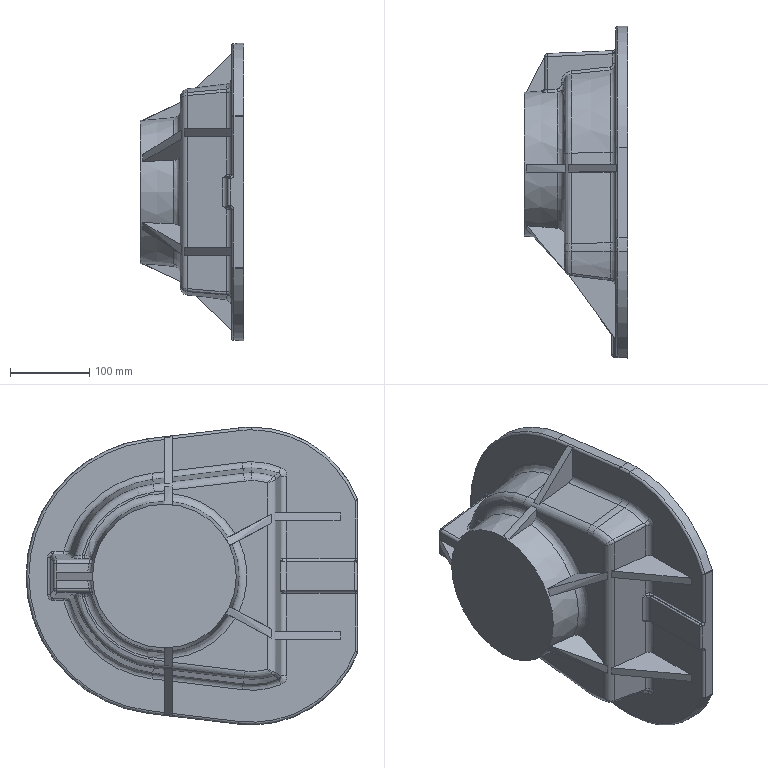Part | STEP file | Input 95 | 1 solid | 162 faces | box 130.5 x 420 x 377 mm | volume 7494076 mm3 | plane 50 | spline 41 | cylinder 33 | torus 25 | cone 11 | sphere 2 | commonest cylinder face diameters 8 x10 16 x9 6 x7 4 x4 20 x3